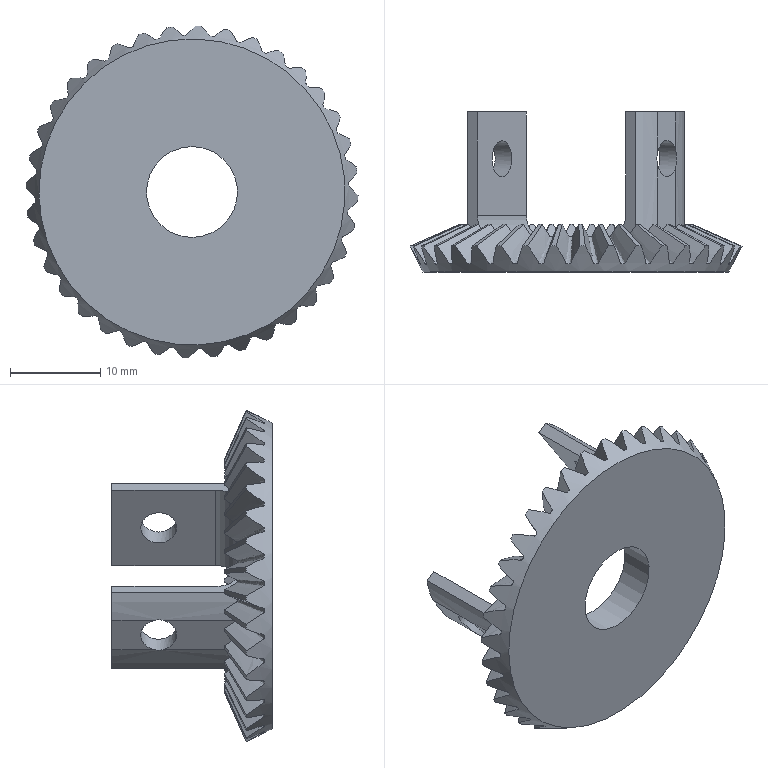Part | STEP file | Zaokr_glenie1 | 1 solid | 100 faces | box 36.885 x 17.8 x 36.885 mm | volume 3718 mm3 | spline 70 | plane 16 | cylinder 10 | cone 4 | commonest cylinder face diameters 24.384 x4 5 x3 4 x2 10.1 x1